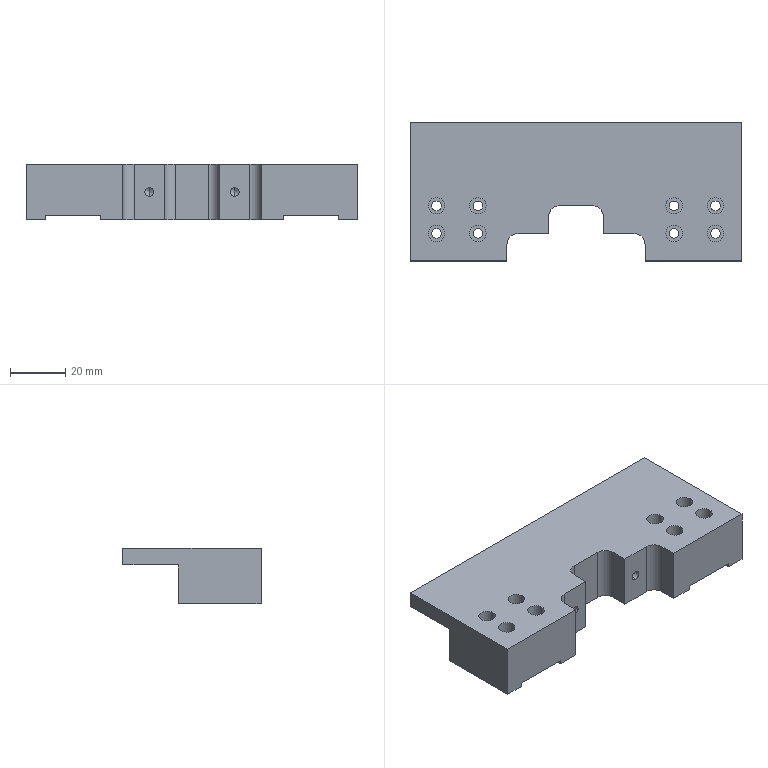Part | SolidWorks | features BaseBody 1 | 1 solid | 84 faces | box 120 x 50 x 20 mm | volume 67533 mm3 | cylinder 44 | plane 32 | cone 8 | commonest cylinder face diameters 3.5 x16 6 x16 3.242 x4 5 x4 8 x4